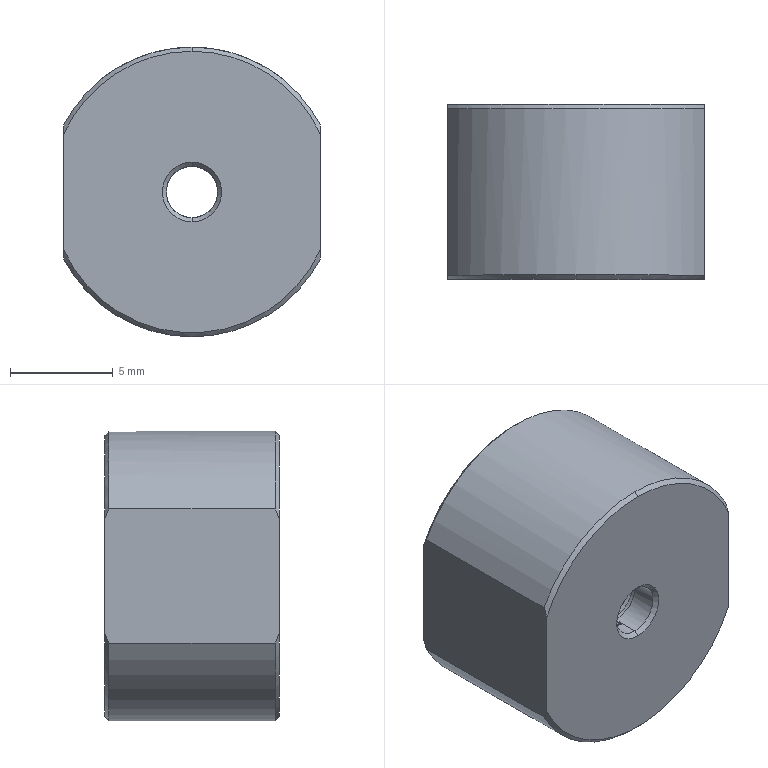Part | SolidWorks | features Chamfer 1, Extrusion 1, Helix 1, SweepCut 1 | 1 solid | 52 faces | box 12.5 x 8.5 x 14.1 mm | volume 1218 mm3 | cylinder 33 | cone 11 | plane 5 | spline 3 | commonest cylinder face diameters 2.5 x30 14.1 x3